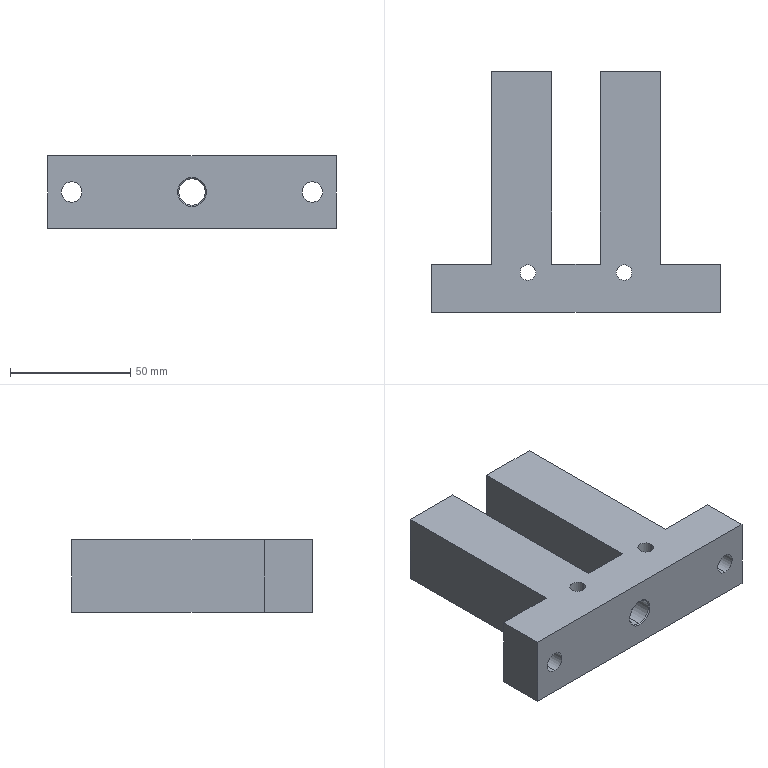Part | STEP file | Pressure plate fixing seat | 1 solid | 60 faces | box 120 x 100 x 30 mm | volume 182269 mm3 | cylinder 22 | cone 20 | plane 18 | commonest cylinder face diameters 11 x6 6.5 x4 6.647 x4 8.5 x4 14 x4